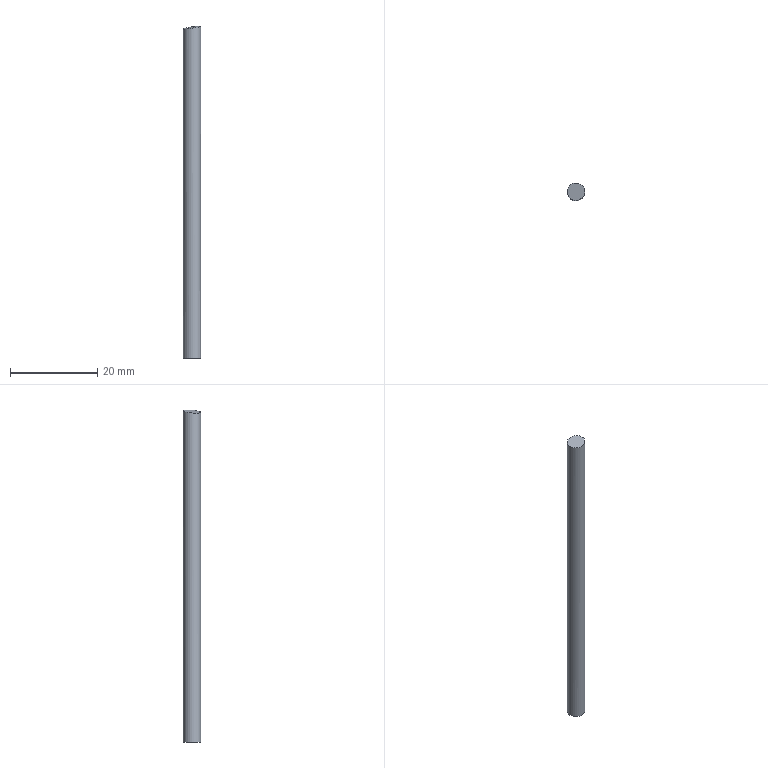Part | NX | features solid 2 | 1 solid | 3 faces | box 4 x 4 x 76.124 mm | volume 951.778 mm3 | plane 1 | cylinder 1 | spline 1 | commonest cylinder face diameters 4 x1
STEP:
#1=CARTESIAN_POINT('',(695.847,-9.202,-80.));
#2=VERTEX_POINT('',#1);
#3=CARTESIAN_POINT('',(694.115,-8.202,-80.));
#4=DIRECTION('',(0.,0.,1.));
#5=DIRECTION('',(0.866,-0.5,0.));
#6=AXIS2_PLACEMENT_3D('',#3,#4,#5);
#7=CIRCLE('',#6,2.);
#8=EDGE_CURVE('',#2,#2,#7,.T.);
#9=ORIENTED_EDGE('',*,*,#8,.F.);
#10=EDGE_LOOP('',(#9));
#11=FACE_BOUND('',#10,.T.);
#12=CARTESIAN_POINT('',(694.115,-8.202,-80.));
#13=DIRECTION('',(0.,0.,1.));
#14=DIRECTION('',(1.,0.,0.));
#15=AXIS2_PLACEMENT_3D('',#12,#13,#14);
#16=PLANE('',#15);
#17=ADVANCED_FACE('',(#11),#16,.F.);
#18=CARTESIAN_POINT('',(692.115,-8.202,-4.565));
#19=VERTEX_POINT('',#18);
#20=CARTESIAN_POINT('',(692.557,-9.785,-4.622));
#21=CARTESIAN_POINT('',(691.895,-8.198,-4.6));
#22=CARTESIAN_POINT('',(692.552,-6.636,-4.368));
#23=CARTESIAN_POINT('',(694.096,-5.99,-4.066));
#24=CARTESIAN_POINT('',(695.672,-6.619,-3.859));
#25=CARTESIAN_POINT('',(696.334,-8.206,-3.877));
#26=CARTESIAN_POINT('',(695.679,-9.766,-4.112));
#27=CARTESIAN_POINT('',(694.136,-10.415,-4.417));
#28=CARTESIAN_POINT('',(692.557,-9.785,-4.622));
#29=CARTESIAN_POINT('',(691.895,-8.198,-4.6));
#30=CARTESIAN_POINT('',(692.552,-6.636,-4.368));
#31=B_SPLINE_CURVE_WITH_KNOTS('',3,(#20,#21,#22,#23,#24,#25,#26,#27,#28,#29,#30),.UNSPECIFIED.,.T.,.F.,(1,1,1,1,1,1,1,1,1,1,1,1,1,1,1),(-0.004727,-0.003152,-0.001576,0.,0.001576,0.003152,0.004727,0.006303,0.007879,0.009455,0.01103,0.01261,0.01418,0.01576,0.01733),.UNSPECIFIED.);
#32=EDGE_CURVE('',#19,#19,#31,.T.);
#33=ORIENTED_EDGE('',*,*,#32,.T.);
#34=EDGE_LOOP('',(#33));
#35=FACE_BOUND('',#34,.T.);
#36=ORIENTED_EDGE('',*,*,#8,.T.);
#37=EDGE_LOOP('',(#36));
#38=FACE_BOUND('',#37,.T.);
#39=CARTESIAN_POINT('',(694.115,-8.202,420.));
#40=DIRECTION('',(0.,0.,-1.));
#41=DIRECTION('',(-1.,0.,0.));
#42=AXIS2_PLACEMENT_3D('',#39,#40,#41);
#43=CYLINDRICAL_SURFACE('',#42,2.);
#44=ADVANCED_FACE('',(#35,#38),#43,.T.);
#45=ORIENTED_EDGE('',*,*,#32,.F.);
#46=EDGE_LOOP('',(#45));
#47=FACE_BOUND('',#46,.T.);
#48=CARTESIAN_POINT('',(692.041,-6.187,-4.414));
#49=CARTESIAN_POINT('',(692.135,-10.253,-4.727));
#50=CARTESIAN_POINT('',(693.395,-6.173,-4.196));
#51=CARTESIAN_POINT('',(693.489,-10.239,-4.509));
#52=CARTESIAN_POINT('',(694.749,-6.159,-3.974));
#53=CARTESIAN_POINT('',(694.843,-10.224,-4.287));
#54=CARTESIAN_POINT('',(696.102,-6.145,-3.749));
#55=CARTESIAN_POINT('',(696.196,-10.21,-4.062));
#56=(BOUNDED_SURFACE()B_SPLINE_SURFACE(3,1,((#48,#49),(#50,#51),(#52,#53),(#54,#55)),.CYLINDRICAL_SURF.,.F.,.F.,.F.)B_SPLINE_SURFACE_WITH_KNOTS((4,4),(2,2),(0.8246,0.8556),(0.5592,0.5911),.PIECEWISE_BEZIER_KNOTS.)GEOMETRIC_REPRESENTATION_ITEM()RATIONAL_B_SPLINE_SURFACE(((0.999,0.999),(0.9991,0.9991),(0.9991,0.9991),(0.9992,0.9992)))REPRESENTATION_ITEM('')SURFACE());
#57=ADVANCED_FACE('',(#47),#56,.F.);
#58=CLOSED_SHELL('',(#17,#44,#57));
#59=MANIFOLD_SOLID_BREP('',#58);
#60=(LENGTH_UNIT()NAMED_UNIT(*)SI_UNIT(.MILLI.,.METRE.));
#61=UNCERTAINTY_MEASURE_WITH_UNIT(LENGTH_MEASURE(0.0508),#60,'','');
#62=(NAMED_UNIT(*)PLANE_ANGLE_UNIT()SI_UNIT($,.RADIAN.));
#63=(NAMED_UNIT(*)SI_UNIT($,.STERADIAN.)SOLID_ANGLE_UNIT());
#64=(GEOMETRIC_REPRESENTATION_CONTEXT(3)GLOBAL_UNCERTAINTY_ASSIGNED_CONTEXT((#61))GLOBAL_UNIT_ASSIGNED_CONTEXT((#60,#62,#63))REPRESENTATION_CONTEXT('',''));
#65=ADVANCED_BREP_SHAPE_REPRESENTATION('',(#59),#64);